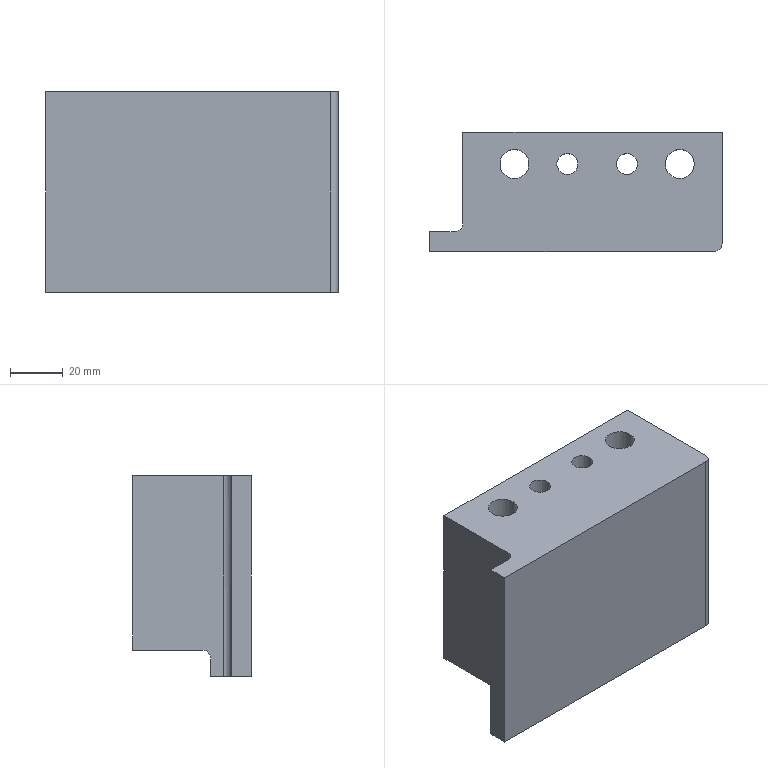Part | NX | features solid 2 | 1 solid | 25 faces | box 110.531 x 45 x 76 mm | volume 282119 mm3 | plane 14 | cylinder 11 | commonest cylinder face diameters 6 x3 8 x2 10.505 x2 11 x2 17 x2
STEP:
#1=CARTESIAN_POINT('',(712.498,169.969,32.999));
#2=VERTEX_POINT('',#1);
#3=CARTESIAN_POINT('',(712.498,166.969,32.999));
#4=VERTEX_POINT('',#3);
#5=CARTESIAN_POINT('',(712.498,196.487,32.999));
#6=DIRECTION('',(0.,-1.,-0.000000517));
#7=VECTOR('',#6,1000.);
#8=LINE('',#5,#7);
#9=EDGE_CURVE('',#2,#4,#8,.T.);
#10=ORIENTED_EDGE('',*,*,#9,.T.);
#11=CARTESIAN_POINT('',(709.498,163.969,32.999));
#12=VERTEX_POINT('',#11);
#13=CARTESIAN_POINT('',(709.498,166.969,32.999));
#14=DIRECTION('',(0.000000053,-0.000000517,1.));
#15=DIRECTION('',(0.01202,0.9999,0.000000516));
#16=AXIS2_PLACEMENT_3D('',#13,#14,#15);
#17=ELLIPSE('',#16,3.,3.);
#18=EDGE_CURVE('',#4,#12,#17,.F.);
#19=ORIENTED_EDGE('',*,*,#18,.T.);
#20=CARTESIAN_POINT('',(699.977,163.969,32.999));
#21=VERTEX_POINT('',#20);
#22=CARTESIAN_POINT('',(704.737,163.969,32.999));
#23=DIRECTION('',(1.,0.,-0.000000053));
#24=VECTOR('',#23,1000.);
#25=LINE('',#22,#24);
#26=EDGE_CURVE('',#12,#21,#25,.F.);
#27=ORIENTED_EDGE('',*,*,#26,.T.);
#28=CARTESIAN_POINT('',(699.977,156.487,32.999));
#29=VERTEX_POINT('',#28);
#30=CARTESIAN_POINT('',(699.977,196.487,32.999));
#31=DIRECTION('',(0.,-1.,-0.000000517));
#32=VECTOR('',#31,1000.);
#33=LINE('',#30,#32);
#34=EDGE_CURVE('',#29,#21,#33,.F.);
#35=ORIENTED_EDGE('',*,*,#34,.F.);
#36=CARTESIAN_POINT('',(807.509,156.487,32.999));
#37=VERTEX_POINT('',#36);
#38=CARTESIAN_POINT('',(699.977,156.487,32.999));
#39=DIRECTION('',(-1.,0.,0.000000053));
#40=VECTOR('',#39,1000.);
#41=LINE('',#38,#40);
#42=EDGE_CURVE('',#29,#37,#41,.F.);
#43=ORIENTED_EDGE('',*,*,#42,.T.);
#44=CARTESIAN_POINT('',(810.509,159.487,32.999));
#45=VERTEX_POINT('',#44);
#46=CARTESIAN_POINT('',(807.509,159.487,32.999));
#47=DIRECTION('',(-0.000000053,0.000000517,-1.));
#48=DIRECTION('',(0.,-1.,-0.000000517));
#49=AXIS2_PLACEMENT_3D('',#46,#47,#48);
#50=CIRCLE('',#49,3.);
#51=EDGE_CURVE('',#45,#37,#50,.T.);
#52=ORIENTED_EDGE('',*,*,#51,.F.);
#53=CARTESIAN_POINT('',(810.509,201.487,32.999));
#54=VERTEX_POINT('',#53);
#55=CARTESIAN_POINT('',(810.509,186.487,32.999));
#56=DIRECTION('',(0.,1.,0.000000517));
#57=VECTOR('',#56,1000.);
#58=LINE('',#55,#57);
#59=EDGE_CURVE('',#54,#45,#58,.F.);
#60=ORIENTED_EDGE('',*,*,#59,.F.);
#61=CARTESIAN_POINT('',(712.498,201.487,32.999));
#62=VERTEX_POINT('',#61);
#63=CARTESIAN_POINT('',(699.977,201.487,32.999));
#64=DIRECTION('',(-1.,0.,0.000000053));
#65=VECTOR('',#64,1000.);
#66=LINE('',#63,#65);
#67=EDGE_CURVE('',#62,#54,#66,.F.);
#68=ORIENTED_EDGE('',*,*,#67,.F.);
#69=CARTESIAN_POINT('',(712.498,196.487,32.999));
#70=DIRECTION('',(0.,1.,0.000000517));
#71=VECTOR('',#70,1000.);
#72=LINE('',#69,#71);
#73=EDGE_CURVE('',#62,#2,#72,.F.);
#74=ORIENTED_EDGE('',*,*,#73,.T.);
#75=EDGE_LOOP('',(#10,#19,#27,#35,#43,#52,#60,#68,#74));
#76=FACE_BOUND('',#75,.T.);
#77=CARTESIAN_POINT('',(794.509,183.987,32.999));
#78=VERTEX_POINT('',#77);
#79=CARTESIAN_POINT('',(794.509,189.487,32.999));
#80=DIRECTION('',(0.000000053,-0.000000517,1.));
#81=DIRECTION('',(0.,-1.,-0.000000517));
#82=AXIS2_PLACEMENT_3D('',#79,#80,#81);
#83=CIRCLE('',#82,5.5);
#84=EDGE_CURVE('',#78,#78,#83,.T.);
#85=ORIENTED_EDGE('',*,*,#84,.F.);
#86=EDGE_LOOP('',(#85));
#87=FACE_BOUND('',#86,.T.);
#88=CARTESIAN_POINT('',(731.977,183.987,32.999));
#89=VERTEX_POINT('',#88);
#90=CARTESIAN_POINT('',(731.977,189.487,32.999));
#91=DIRECTION('',(0.000000053,-0.000000517,1.));
#92=DIRECTION('',(0.,-1.,-0.000000517));
#93=AXIS2_PLACEMENT_3D('',#90,#91,#92);
#94=CIRCLE('',#93,5.5);
#95=EDGE_CURVE('',#89,#89,#94,.T.);
#96=ORIENTED_EDGE('',*,*,#95,.F.);
#97=EDGE_LOOP('',(#96));
#98=FACE_BOUND('',#97,.T.);
#99=CARTESIAN_POINT('',(774.509,193.487,32.999));
#100=VERTEX_POINT('',#99);
#101=CARTESIAN_POINT('',(774.509,189.487,32.999));
#102=DIRECTION('',(0.000000053,-0.000000517,1.));
#103=DIRECTION('',(0.,1.,0.000000517));
#104=AXIS2_PLACEMENT_3D('',#101,#102,#103);
#105=CIRCLE('',#104,4.);
#106=EDGE_CURVE('',#100,#100,#105,.T.);
#107=ORIENTED_EDGE('',*,*,#106,.F.);
#108=EDGE_LOOP('',(#107));
#109=FACE_BOUND('',#108,.T.);
#110=CARTESIAN_POINT('',(751.977,193.487,32.999));
#111=VERTEX_POINT('',#110);
#112=CARTESIAN_POINT('',(751.977,189.487,32.999));
#113=DIRECTION('',(0.000000053,-0.000000517,1.));
#114=DIRECTION('',(0.,1.,0.000000517));
#115=AXIS2_PLACEMENT_3D('',#112,#113,#114);
#116=CIRCLE('',#115,4.);
#117=EDGE_CURVE('',#111,#111,#116,.T.);
#118=ORIENTED_EDGE('',*,*,#117,.F.);
#119=EDGE_LOOP('',(#118));
#120=FACE_BOUND('',#119,.T.);
#121=CARTESIAN_POINT('',(699.977,196.487,32.999));
#122=DIRECTION('',(0.000000053,-0.000000517,1.));
#123=DIRECTION('',(1.,0.,-0.000000053));
#124=AXIS2_PLACEMENT_3D('',#121,#122,#123);
#125=PLANE('',#124);
#126=ADVANCED_FACE('',(#76,#87,#98,#109,#120),#125,.T.);
#127=CARTESIAN_POINT('',(794.509,197.987,-33.001));
#128=VERTEX_POINT('',#127);
#129=CARTESIAN_POINT('',(794.509,189.487,-33.001));
#130=DIRECTION('',(-0.000000053,0.000000517,-1.));
#131=DIRECTION('',(0.,1.,0.000000517));
#132=AXIS2_PLACEMENT_3D('',#129,#130,#131);
#133=CIRCLE('',#132,8.5);
#134=EDGE_CURVE('',#128,#128,#133,.F.);
#135=ORIENTED_EDGE('',*,*,#134,.T.);
#136=EDGE_LOOP('',(#135));
#137=FACE_BOUND('',#136,.T.);
#138=CARTESIAN_POINT('',(774.509,184.234,-33.001));
#139=VERTEX_POINT('',#138);
#140=CARTESIAN_POINT('',(773.441,184.308,-33.001));
#141=CARTESIAN_POINT('',(774.473,184.201,-33.001));
#142=CARTESIAN_POINT('',(775.504,184.297,-33.001));
#143=CARTESIAN_POINT('',(776.482,184.583,-33.001));
#144=CARTESIAN_POINT('',(777.4,185.061,-33.001));
#145=CARTESIAN_POINT('',(778.208,185.71,-33.001));
#146=CARTESIAN_POINT('',(778.873,186.505,-33.001));
#147=CARTESIAN_POINT('',(779.371,187.413,-33.001));
#148=CARTESIAN_POINT('',(779.682,188.402,-33.001));
#149=CARTESIAN_POINT('',(779.795,189.432,-33.001));
#150=CARTESIAN_POINT('',(779.704,190.464,-33.001));
#151=CARTESIAN_POINT('',(779.413,191.459,-33.001));
#152=CARTESIAN_POINT('',(778.934,192.378,-33.001));
#153=CARTESIAN_POINT('',(778.285,193.186,-33.001));
#154=CARTESIAN_POINT('',(777.491,193.852,-33.001));
#155=CARTESIAN_POINT('',(776.582,194.35,-33.001));
#156=CARTESIAN_POINT('',(775.594,194.661,-33.001));
#157=CARTESIAN_POINT('',(774.563,194.773,-33.001));
#158=CARTESIAN_POINT('',(773.531,194.682,-33.001));
#159=CARTESIAN_POINT('',(772.536,194.392,-33.001));
#160=CARTESIAN_POINT('',(771.617,193.913,-33.001));
#161=CARTESIAN_POINT('',(770.81,193.264,-33.001));
#162=CARTESIAN_POINT('',(770.144,192.469,-33.001));
#163=CARTESIAN_POINT('',(769.646,191.561,-33.001));
#164=CARTESIAN_POINT('',(769.335,190.572,-33.001));
#165=CARTESIAN_POINT('',(769.223,189.542,-33.001));
#166=CARTESIAN_POINT('',(769.313,188.509,-33.001));
#167=CARTESIAN_POINT('',(769.604,187.515,-33.001));
#168=CARTESIAN_POINT('',(770.083,186.596,-33.001));
#169=CARTESIAN_POINT('',(770.732,185.788,-33.001));
#170=CARTESIAN_POINT('',(771.526,185.122,-33.001));
#171=CARTESIAN_POINT('',(772.435,184.624,-33.001));
#172=CARTESIAN_POINT('',(773.441,184.308,-33.001));
#173=CARTESIAN_POINT('',(774.473,184.201,-33.001));
#174=CARTESIAN_POINT('',(775.504,184.297,-33.001));
#175=B_SPLINE_CURVE_WITH_KNOTS('',3,(#140,#141,#142,#143,#144,#145,#146,#147,#148,#149,#150,#151,#152,#153,#154,#155,#156,#157,#158,#159,#160,#161,#162,#163,#164,#165,#166,#167,#168,#169,#170,#171,#172,#173,#174),.UNSPECIFIED.,.T.,.F.,(1,1,1,1,1,1,1,1,1,1,1,1,1,1,1,1,1,1,1,1,1,1,1,1,1,1,1,1,1,1,1,1,1,1,1,1,1,1,1),(-0.09539,-0.06414,-0.03289,0.,0.02969,0.06086,0.09211,0.1234,0.1546,0.1859,0.2171,0.2484,0.2796,0.3109,0.3421,0.3734,0.4046,0.4359,0.4671,0.4984,0.5296,0.5609,0.5921,0.6234,0.6546,0.6859,0.7171,0.7484,0.7796,0.8109,0.8421,0.8734,0.9046,0.9359,0.9671,1.,1.03,1.061,1.092),.UNSPECIFIED.);
#176=EDGE_CURVE('',#139,#139,#175,.T.);
#177=ORIENTED_EDGE('',*,*,#176,.T.);
#178=EDGE_LOOP('',(#177));
#179=FACE_BOUND('',#178,.T.);
#180=CARTESIAN_POINT('',(751.977,184.234,-33.001));
#181=VERTEX_POINT('',#180);
#182=CARTESIAN_POINT('',(750.91,184.308,-33.001));
#183=CARTESIAN_POINT('',(751.942,184.201,-33.001));
#184=CARTESIAN_POINT('',(752.973,184.297,-33.001));
#185=CARTESIAN_POINT('',(753.95,184.583,-33.001));
#186=CARTESIAN_POINT('',(754.869,185.061,-33.001));
#187=CARTESIAN_POINT('',(755.676,185.71,-33.001));
#188=CARTESIAN_POINT('',(756.342,186.505,-33.001));
#189=CARTESIAN_POINT('',(756.84,187.413,-33.001));
#190=CARTESIAN_POINT('',(757.151,188.402,-33.001));
#191=CARTESIAN_POINT('',(757.263,189.432,-33.001));
#192=CARTESIAN_POINT('',(757.172,190.464,-33.001));
#193=CARTESIAN_POINT('',(756.882,191.459,-33.001));
#194=CARTESIAN_POINT('',(756.403,192.378,-33.001));
#195=CARTESIAN_POINT('',(755.754,193.186,-33.001));
#196=CARTESIAN_POINT('',(754.96,193.852,-33.001));
#197=CARTESIAN_POINT('',(754.051,194.35,-33.001));
#198=CARTESIAN_POINT('',(753.062,194.661,-33.001));
#199=CARTESIAN_POINT('',(752.032,194.773,-33.001));
#200=CARTESIAN_POINT('',(751.,194.682,-33.001));
#201=CARTESIAN_POINT('',(750.005,194.392,-33.001));
#202=CARTESIAN_POINT('',(749.086,193.913,-33.001));
#203=CARTESIAN_POINT('',(748.278,193.264,-33.001));
#204=CARTESIAN_POINT('',(747.613,192.469,-33.001));
#205=CARTESIAN_POINT('',(747.115,191.561,-33.001));
#206=CARTESIAN_POINT('',(746.803,190.572,-33.001));
#207=CARTESIAN_POINT('',(746.691,189.542,-33.001));
#208=CARTESIAN_POINT('',(746.782,188.51,-33.001));
#209=CARTESIAN_POINT('',(747.073,187.515,-33.001));
#210=CARTESIAN_POINT('',(747.552,186.596,-33.001));
#211=CARTESIAN_POINT('',(748.201,185.788,-33.001));
#212=CARTESIAN_POINT('',(748.995,185.122,-33.001));
#213=CARTESIAN_POINT('',(749.904,184.624,-33.001));
#214=CARTESIAN_POINT('',(750.91,184.308,-33.001));
#215=CARTESIAN_POINT('',(751.942,184.201,-33.001));
#216=CARTESIAN_POINT('',(752.973,184.297,-33.001));
#217=B_SPLINE_CURVE_WITH_KNOTS('',3,(#182,#183,#184,#185,#186,#187,#188,#189,#190,#191,#192,#193,#194,#195,#196,#197,#198,#199,#200,#201,#202,#203,#204,#205,#206,#207,#208,#209,#210,#211,#212,#213,#214,#215,#216),.UNSPECIFIED.,.T.,.F.,(1,1,1,1,1,1,1,1,1,1,1,1,1,1,1,1,1,1,1,1,1,1,1,1,1,1,1,1,1,1,1,1,1,1,1,1,1,1,1),(-0.09539,-0.06414,-0.03289,0.,0.02969,0.06086,0.09211,0.1234,0.1546,0.1859,0.2171,0.2484,0.2796,0.3109,0.3421,0.3734,0.4046,0.4359,0.4671,0.4984,0.5296,0.5609,0.5921,0.6234,0.6546,0.6859,0.7171,0.7484,0.7796,0.8109,0.8421,0.8734,0.9046,0.9359,0.9671,1.,1.03,1.061,1.092),.UNSPECIFIED.);
#218=EDGE_CURVE('',#181,#181,#217,.T.);
#219=ORIENTED_EDGE('',*,*,#218,.T.);
#220=EDGE_LOOP('',(#219));
#221=FACE_BOUND('',#220,.T.);
#222=CARTESIAN_POINT('',(731.977,197.987,-33.001));
#223=VERTEX_POINT('',#222);
#224=CARTESIAN_POINT('',(731.977,189.487,-33.001));
#225=DIRECTION('',(-0.000000053,0.000000517,-1.));
#226=DIRECTION('',(0.,1.,0.000000517));
#227=AXIS2_PLACEMENT_3D('',#224,#225,#226);
#228=CIRCLE('',#227,8.5);
#229=EDGE_CURVE('',#223,#223,#228,.F.);
#230=ORIENTED_EDGE('',*,*,#229,.T.);
#231=EDGE_LOOP('',(#230));
#232=FACE_BOUND('',#231,.T.);
#233=CARTESIAN_POINT('',(810.509,201.487,-33.001));
#234=VERTEX_POINT('',#233);
#235=CARTESIAN_POINT('',(810.509,174.969,-33.001));
#236=VERTEX_POINT('',#235);
#237=CARTESIAN_POINT('',(810.509,186.487,-33.001));
#238=DIRECTION('',(0.,-1.,-0.000000517));
#239=VECTOR('',#238,1000.);
#240=LINE('',#237,#239);
#241=EDGE_CURVE('',#234,#236,#240,.T.);
#242=ORIENTED_EDGE('',*,*,#241,.T.);
#243=CARTESIAN_POINT('',(712.498,174.969,-33.001));
#244=VERTEX_POINT('',#243);
#245=CARTESIAN_POINT('',(712.498,174.969,-33.001));
#246=DIRECTION('',(1.,0.,-0.000000053));
#247=VECTOR('',#246,1000.);
#248=LINE('',#245,#247);
#249=EDGE_CURVE('',#236,#244,#248,.F.);
#250=ORIENTED_EDGE('',*,*,#249,.T.);
#251=CARTESIAN_POINT('',(712.498,201.487,-33.001));
#252=VERTEX_POINT('',#251);
#253=CARTESIAN_POINT('',(712.498,119.199,-33.001));
#254=DIRECTION('',(0.,-1.,-0.000000517));
#255=VECTOR('',#254,1000.);
#256=LINE('',#253,#255);
#257=EDGE_CURVE('',#252,#244,#256,.T.);
#258=ORIENTED_EDGE('',*,*,#257,.F.);
#259=CARTESIAN_POINT('',(574.977,201.487,-33.001));
#260=DIRECTION('',(-1.,0.,0.000000053));
#261=VECTOR('',#260,1000.);
#262=LINE('',#259,#261);
#263=EDGE_CURVE('',#234,#252,#262,.T.);
#264=ORIENTED_EDGE('',*,*,#263,.F.);
#265=EDGE_LOOP('',(#242,#250,#258,#264));
#266=FACE_BOUND('',#265,.T.);
#267=CARTESIAN_POINT('',(574.977,119.199,-33.001));
#268=DIRECTION('',(-0.000000053,0.000000517,-1.));
#269=DIRECTION('',(1.,0.,-0.000000053));
#270=AXIS2_PLACEMENT_3D('',#267,#268,#269);
#271=PLANE('',#270);
#272=ADVANCED_FACE('',(#137,#179,#221,#232,#266),#271,.T.);
#273=CARTESIAN_POINT('',(712.498,171.969,-36.001));
#274=VERTEX_POINT('',#273);
#275=CARTESIAN_POINT('',(712.498,171.969,-43.001));
#276=VERTEX_POINT('',#275);
#277=CARTESIAN_POINT('',(712.498,171.969,49.2));
#278=DIRECTION('',(0.,0.000001782,-1.));
#279=VECTOR('',#278,1000.);
#280=LINE('',#277,#279);
#281=EDGE_CURVE('',#274,#276,#280,.T.);
#282=ORIENTED_EDGE('',*,*,#281,.F.);
#283=CARTESIAN_POINT('',(810.509,171.969,-36.001));
#284=VERTEX_POINT('',#283);
#285=CARTESIAN_POINT('',(810.509,171.969,-36.001));
#286=DIRECTION('',(1.,0.,-0.000000053));
#287=VECTOR('',#286,1000.);
#288=LINE('',#285,#287);
#289=EDGE_CURVE('',#274,#284,#288,.T.);
#290=ORIENTED_EDGE('',*,*,#289,.T.);
#291=CARTESIAN_POINT('',(810.509,171.969,-43.001));
#292=VERTEX_POINT('',#291);
#293=CARTESIAN_POINT('',(810.509,171.969,-43.001));
#294=DIRECTION('',(0.000000053,-0.000001782,1.));
#295=VECTOR('',#294,1000.);
#296=LINE('',#293,#295);
#297=EDGE_CURVE('',#292,#284,#296,.T.);
#298=ORIENTED_EDGE('',*,*,#297,.F.);
#299=CARTESIAN_POINT('',(704.737,171.969,-43.001));
#300=DIRECTION('',(-1.,0.,0.000000053));
#301=VECTOR('',#300,1000.);
#302=LINE('',#299,#301);
#303=EDGE_CURVE('',#292,#276,#302,.T.);
#304=ORIENTED_EDGE('',*,*,#303,.T.);
#305=EDGE_LOOP('',(#282,#290,#298,#304));
#306=FACE_BOUND('',#305,.T.);
#307=CARTESIAN_POINT('',(704.737,171.969,-5.001));
#308=DIRECTION('',(0.,1.,0.000001782));
#309=DIRECTION('',(0.,0.000001782,-1.));
#310=AXIS2_PLACEMENT_3D('',#307,#308,#309);
#311=PLANE('',#310);
#312=ADVANCED_FACE('',(#306),#311,.T.);
#313=ORIENTED_EDGE('',*,*,#42,.F.);
#314=CARTESIAN_POINT('',(699.977,156.487,-43.001));
#315=VERTEX_POINT('',#314);
#316=CARTESIAN_POINT('',(699.977,156.487,56.368));
#317=DIRECTION('',(0.000000053,-0.000000517,1.));
#318=VECTOR('',#317,1000.);
#319=LINE('',#316,#318);
#320=EDGE_CURVE('',#29,#315,#319,.F.);
#321=ORIENTED_EDGE('',*,*,#320,.T.);
#322=CARTESIAN_POINT('',(807.509,156.487,-43.001));
#323=VERTEX_POINT('',#322);
#324=CARTESIAN_POINT('',(574.977,156.487,-43.001));
#325=DIRECTION('',(1.,0.,-0.000000053));
#326=VECTOR('',#325,1000.);
#327=LINE('',#324,#326);
#328=EDGE_CURVE('',#315,#323,#327,.T.);
#329=ORIENTED_EDGE('',*,*,#328,.T.);
#330=CARTESIAN_POINT('',(807.509,156.487,56.368));
#331=DIRECTION('',(-0.000000053,0.000000517,-1.));
#332=VECTOR('',#331,1000.);
#333=LINE('',#330,#332);
#334=EDGE_CURVE('',#323,#37,#333,.F.);
#335=ORIENTED_EDGE('',*,*,#334,.T.);
#336=EDGE_LOOP('',(#313,#321,#329,#335));
#337=FACE_BOUND('',#336,.T.);
#338=CARTESIAN_POINT('',(583.446,156.487,56.368));
#339=DIRECTION('',(0.,1.,0.000000517));
#340=DIRECTION('',(-0.000000053,0.000000517,-1.));
#341=AXIS2_PLACEMENT_3D('',#338,#339,#340);
#342=PLANE('',#341);
#343=ADVANCED_FACE('',(#337),#342,.F.);
#344=ORIENTED_EDGE('',*,*,#328,.F.);
#345=CARTESIAN_POINT('',(699.977,163.969,-43.001));
#346=VERTEX_POINT('',#345);
#347=CARTESIAN_POINT('',(699.977,119.199,-43.001));
#348=DIRECTION('',(0.,1.,0.000000517));
#349=VECTOR('',#348,1000.);
#350=LINE('',#347,#349);
#351=EDGE_CURVE('',#346,#315,#350,.F.);
#352=ORIENTED_EDGE('',*,*,#351,.F.);
#353=CARTESIAN_POINT('',(709.498,163.969,-43.001));
#354=VERTEX_POINT('',#353);
#355=CARTESIAN_POINT('',(704.737,163.969,-43.001));
#356=DIRECTION('',(-1.,0.,0.000000053));
#357=VECTOR('',#356,1000.);
#358=LINE('',#355,#357);
#359=EDGE_CURVE('',#354,#346,#358,.T.);
#360=ORIENTED_EDGE('',*,*,#359,.F.);
#361=CARTESIAN_POINT('',(712.498,166.969,-43.001));
#362=VERTEX_POINT('',#361);
#363=CARTESIAN_POINT('',(709.498,166.969,-43.001));
#364=DIRECTION('',(-0.000000053,0.000000517,-1.));
#365=DIRECTION('',(0.01202,0.9999,0.000000516));
#366=AXIS2_PLACEMENT_3D('',#363,#364,#365);
#367=ELLIPSE('',#366,3.,3.);
#368=EDGE_CURVE('',#354,#362,#367,.F.);
#369=ORIENTED_EDGE('',*,*,#368,.T.);
#370=CARTESIAN_POINT('',(712.498,119.199,-43.001));
#371=DIRECTION('',(0.,1.,0.000000517));
#372=VECTOR('',#371,1000.);
#373=LINE('',#370,#372);
#374=EDGE_CURVE('',#362,#276,#373,.T.);
#375=ORIENTED_EDGE('',*,*,#374,.T.);
#376=ORIENTED_EDGE('',*,*,#303,.F.);
#377=CARTESIAN_POINT('',(810.509,159.487,-43.001));
#378=VERTEX_POINT('',#377);
#379=CARTESIAN_POINT('',(810.509,186.487,-43.001));
#380=DIRECTION('',(0.,-1.,-0.000000517));
#381=VECTOR('',#380,1000.);
#382=LINE('',#379,#381);
#383=EDGE_CURVE('',#292,#378,#382,.T.);
#384=ORIENTED_EDGE('',*,*,#383,.T.);
#385=CARTESIAN_POINT('',(807.509,159.487,-43.001));
#386=DIRECTION('',(0.000000053,-0.000000517,1.));
#387=DIRECTION('',(0.,1.,0.000000517));
#388=AXIS2_PLACEMENT_3D('',#385,#386,#387);
#389=CIRCLE('',#388,3.);
#390=EDGE_CURVE('',#378,#323,#389,.F.);
#391=ORIENTED_EDGE('',*,*,#390,.T.);
#392=EDGE_LOOP('',(#344,#352,#360,#369,#375,#376,#384,#391));
#393=FACE_BOUND('',#392,.T.);
#394=CARTESIAN_POINT('',(574.977,119.199,-43.001));
#395=DIRECTION('',(-0.000000053,0.000000517,-1.));
#396=DIRECTION('',(1.,0.,-0.000000053));
#397=AXIS2_PLACEMENT_3D('',#394,#395,#396);
#398=PLANE('',#397);
#399=ADVANCED_FACE('',(#393),#398,.T.);
#400=ORIENTED_EDGE('',*,*,#59,.T.);
#401=CARTESIAN_POINT('',(810.509,159.487,-43.001));
#402=DIRECTION('',(-0.000000053,0.000000517,-1.));
#403=VECTOR('',#402,1000.);
#404=LINE('',#401,#403);
#405=EDGE_CURVE('',#45,#378,#404,.T.);
#406=ORIENTED_EDGE('',*,*,#405,.T.);
#407=ORIENTED_EDGE('',*,*,#383,.F.);
#408=ORIENTED_EDGE('',*,*,#297,.T.);
#409=CARTESIAN_POINT('',(810.509,174.969,-36.001));
#410=DIRECTION('',(1.,0.,-0.000000053));
#411=DIRECTION('',(-0.000000053,0.,-1.));
#412=AXIS2_PLACEMENT_3D('',#409,#410,#411);
#413=CIRCLE('',#412,3.);
#414=EDGE_CURVE('',#284,#236,#413,.F.);
#415=ORIENTED_EDGE('',*,*,#414,.T.);
#416=ORIENTED_EDGE('',*,*,#241,.F.);
#417=CARTESIAN_POINT('',(810.509,201.487,-43.001));
#418=DIRECTION('',(0.000000053,-0.000000517,1.));
#419=VECTOR('',#418,1000.);
#420=LINE('',#417,#419);
#421=EDGE_CURVE('',#54,#234,#420,.F.);
#422=ORIENTED_EDGE('',*,*,#421,.F.);
#423=EDGE_LOOP('',(#400,#406,#407,#408,#415,#416,#422));
#424=FACE_BOUND('',#423,.T.);
#425=CARTESIAN_POINT('',(810.509,186.487,-43.001));
#426=DIRECTION('',(1.,0.,-0.000000053));
#427=DIRECTION('',(0.000000053,-0.000000517,1.));
#428=AXIS2_PLACEMENT_3D('',#425,#426,#427);
#429=PLANE('',#428);
#430=ADVANCED_FACE('',(#424),#429,.T.);
#431=ORIENTED_EDGE('',*,*,#67,.T.);
#432=ORIENTED_EDGE('',*,*,#421,.T.);
#433=ORIENTED_EDGE('',*,*,#263,.T.);
#434=CARTESIAN_POINT('',(712.498,201.487,-43.001));
#435=DIRECTION('',(0.,0.000000517,-1.));
#436=VECTOR('',#435,1000.);
#437=LINE('',#434,#436);
#438=EDGE_CURVE('',#62,#252,#437,.T.);
#439=ORIENTED_EDGE('',*,*,#438,.F.);
#440=EDGE_LOOP('',(#431,#432,#433,#439));
#441=FACE_BOUND('',#440,.T.);
#442=CARTESIAN_POINT('',(699.977,201.487,-43.001));
#443=DIRECTION('',(0.,1.,0.000000517));
#444=DIRECTION('',(-0.000000053,0.000000517,-1.));
#445=AXIS2_PLACEMENT_3D('',#442,#443,#444);
#446=PLANE('',#445);
#447=ADVANCED_FACE('',(#441),#446,.T.);
#448=ORIENTED_EDGE('',*,*,#257,.T.);
#449=CARTESIAN_POINT('',(712.498,174.969,-36.001));
#450=DIRECTION('',(-1.,0.,0.));
#451=DIRECTION('',(0.,-1.,0.));
#452=AXIS2_PLACEMENT_3D('',#449,#450,#451);
#453=CIRCLE('',#452,3.);
#454=EDGE_CURVE('',#244,#274,#453,.F.);
#455=ORIENTED_EDGE('',*,*,#454,.T.);
#456=ORIENTED_EDGE('',*,*,#281,.T.);
#457=ORIENTED_EDGE('',*,*,#374,.F.);
#458=CARTESIAN_POINT('',(712.498,166.969,32.999));
#459=DIRECTION('',(0.,-0.000004945,1.));
#460=VECTOR('',#459,1000.);
#461=LINE('',#458,#460);
#462=EDGE_CURVE('',#362,#4,#461,.T.);
#463=ORIENTED_EDGE('',*,*,#462,.T.);
#464=ORIENTED_EDGE('',*,*,#9,.F.);
#465=ORIENTED_EDGE('',*,*,#73,.F.);
#466=ORIENTED_EDGE('',*,*,#438,.T.);
#467=EDGE_LOOP('',(#448,#455,#456,#457,#463,#464,#465,#466));
#468=FACE_BOUND('',#467,.T.);
#469=CARTESIAN_POINT('',(712.498,185.969,49.2));
#470=DIRECTION('',(-1.,0.,0.));
#471=DIRECTION('',(0.,1.,0.000004363));
#472=AXIS2_PLACEMENT_3D('',#469,#470,#471);
#473=PLANE('',#472);
#474=ADVANCED_FACE('',(#468),#473,.T.);
#475=CARTESIAN_POINT('',(794.509,194.987,7.999));
#476=VERTEX_POINT('',#475);
#477=CARTESIAN_POINT('',(794.509,189.487,7.999));
#478=DIRECTION('',(-0.00000016,0.000000517,-1.));
#479=DIRECTION('',(0.,1.,0.000000517));
#480=AXIS2_PLACEMENT_3D('',#477,#478,#479);
#481=CIRCLE('',#480,5.5);
#482=EDGE_CURVE('',#476,#476,#481,.F.);
#483=ORIENTED_EDGE('',*,*,#482,.F.);
#484=EDGE_LOOP('',(#483));
#485=FACE_BOUND('',#484,.T.);
#486=ORIENTED_EDGE('',*,*,#84,.T.);
#487=EDGE_LOOP('',(#486));
#488=FACE_BOUND('',#487,.T.);
#489=CARTESIAN_POINT('',(794.509,189.487,33.999));
#490=DIRECTION('',(-0.00000016,0.000000517,-1.));
#491=DIRECTION('',(0.,1.,0.000000517));
#492=AXIS2_PLACEMENT_3D('',#489,#490,#491);
#493=CYLINDRICAL_SURFACE('',#492,5.5);
#494=ADVANCED_FACE('',(#485,#488),#493,.F.);
#495=ORIENTED_EDGE('',*,*,#134,.F.);
#496=EDGE_LOOP('',(#495));
#497=FACE_BOUND('',#496,.T.);
#498=CARTESIAN_POINT('',(794.509,197.987,7.999));
#499=VERTEX_POINT('',#498);
#500=CARTESIAN_POINT('',(794.509,189.487,7.999));
#501=DIRECTION('',(-0.00000016,0.000000517,-1.));
#502=DIRECTION('',(0.,1.,0.000000517));
#503=AXIS2_PLACEMENT_3D('',#500,#501,#502);
#504=CIRCLE('',#503,8.5);
#505=EDGE_CURVE('',#499,#499,#504,.T.);
#506=ORIENTED_EDGE('',*,*,#505,.F.);
#507=EDGE_LOOP('',(#506));
#508=FACE_BOUND('',#507,.T.);
#509=CARTESIAN_POINT('',(794.509,189.487,7.999));
#510=DIRECTION('',(-0.00000016,0.000000517,-1.));
#511=DIRECTION('',(0.,1.,0.000000517));
#512=AXIS2_PLACEMENT_3D('',#509,#510,#511);
#513=CYLINDRICAL_SURFACE('',#512,8.5);
#514=ADVANCED_FACE('',(#497,#508),#513,.F.);
#515=ORIENTED_EDGE('',*,*,#482,.T.);
#516=EDGE_LOOP('',(#515));
#517=FACE_BOUND('',#516,.T.);
#518=ORIENTED_EDGE('',*,*,#505,.T.);
#519=EDGE_LOOP('',(#518));
#520=FACE_BOUND('',#519,.T.);
#521=CARTESIAN_POINT('',(794.509,189.487,7.999));
#522=DIRECTION('',(-0.00000016,0.000000517,-1.));
#523=DIRECTION('',(0.,1.,0.000000517));
#524=AXIS2_PLACEMENT_3D('',#521,#522,#523);
#525=PLANE('',#524);
#526=ADVANCED_FACE('',(#517,#520),#525,.T.);
#527=CARTESIAN_POINT('',(778.509,189.487,-13.001));
#528=VERTEX_POINT('',#527);
#529=CARTESIAN_POINT('',(774.509,189.487,-13.001));
#530=DIRECTION('',(0.000000874,-0.000000517,-1.));
#531=DIRECTION('',(1.,0.,0.000000874));
#532=AXIS2_PLACEMENT_3D('',#529,#530,#531);
#533=CIRCLE('',#532,4.);
#534=EDGE_CURVE('',#528,#528,#533,.F.);
#535=ORIENTED_EDGE('',*,*,#534,.F.);
#536=EDGE_LOOP('',(#535));
#537=FACE_BOUND('',#536,.T.);
#538=ORIENTED_EDGE('',*,*,#106,.T.);
#539=EDGE_LOOP('',(#538));
#540=FACE_BOUND('',#539,.T.);
#541=CARTESIAN_POINT('',(774.509,189.487,33.999));
#542=DIRECTION('',(0.000000874,-0.000000517,-1.));
#543=DIRECTION('',(0.,1.,-0.000000517));
#544=AXIS2_PLACEMENT_3D('',#541,#542,#543);
#545=CYLINDRICAL_SURFACE('',#544,4.);
#546=ADVANCED_FACE('',(#537,#540),#545,.F.);
#547=ORIENTED_EDGE('',*,*,#176,.F.);
#548=EDGE_LOOP('',(#547));
#549=FACE_BOUND('',#548,.T.);
#550=CARTESIAN_POINT('',(779.761,189.487,-13.001));
#551=VERTEX_POINT('',#550);
#552=CARTESIAN_POINT('',(774.509,189.487,-13.001));
#553=DIRECTION('',(0.000000874,-0.000000517,-1.));
#554=DIRECTION('',(1.,0.,0.000000874));
#555=AXIS2_PLACEMENT_3D('',#552,#553,#554);
#556=CIRCLE('',#555,5.253);
#557=EDGE_CURVE('',#551,#551,#556,.T.);
#558=ORIENTED_EDGE('',*,*,#557,.F.);
#559=EDGE_LOOP('',(#558));
#560=FACE_BOUND('',#559,.T.);
#561=CARTESIAN_POINT('',(774.509,189.487,-33.001));
#562=DIRECTION('',(0.000000874,-0.000000517,-1.));
#563=DIRECTION('',(0.,1.,-0.000000517));
#564=AXIS2_PLACEMENT_3D('',#561,#562,#563);
#565=CYLINDRICAL_SURFACE('',#564,5.253);
#566=ADVANCED_FACE('',(#549,#560),#565,.F.);
#567=ORIENTED_EDGE('',*,*,#534,.T.);
#568=EDGE_LOOP('',(#567));
#569=FACE_BOUND('',#568,.T.);
#570=ORIENTED_EDGE('',*,*,#557,.T.);
#571=EDGE_LOOP('',(#570));
#572=FACE_BOUND('',#571,.T.);
#573=CARTESIAN_POINT('',(774.509,189.487,-13.001));
#574=DIRECTION('',(0.000000874,-0.000000517,-1.));
#575=DIRECTION('',(0.,1.,-0.000000517));
#576=AXIS2_PLACEMENT_3D('',#573,#574,#575);
#577=PLANE('',#576);
#578=ADVANCED_FACE('',(#569,#572),#577,.T.);
#579=CARTESIAN_POINT('',(751.977,193.487,-13.001));
#580=VERTEX_POINT('',#579);
#581=CARTESIAN_POINT('',(751.977,189.487,-13.001));
#582=DIRECTION('',(-0.000001087,-0.000000517,-1.));
#583=DIRECTION('',(0.,1.,-0.000000517));
#584=AXIS2_PLACEMENT_3D('',#581,#582,#583);
#585=CIRCLE('',#584,4.);
#586=EDGE_CURVE('',#580,#580,#585,.T.);
#587=ORIENTED_EDGE('',*,*,#586,.T.);
#588=EDGE_LOOP('',(#587));
#589=FACE_BOUND('',#588,.T.);
#590=ORIENTED_EDGE('',*,*,#117,.T.);
#591=EDGE_LOOP('',(#590));
#592=FACE_BOUND('',#591,.T.);
#593=CARTESIAN_POINT('',(751.977,189.487,33.999));
#594=DIRECTION('',(-0.000001087,-0.000000517,-1.));
#595=DIRECTION('',(0.,1.,-0.000000517));
#596=AXIS2_PLACEMENT_3D('',#593,#594,#595);
#597=CYLINDRICAL_SURFACE('',#596,4.);
#598=ADVANCED_FACE('',(#589,#592),#597,.F.);
#599=ORIENTED_EDGE('',*,*,#218,.F.);
#600=EDGE_LOOP('',(#599));
#601=FACE_BOUND('',#600,.T.);
#602=CARTESIAN_POINT('',(746.725,189.487,-13.001));
#603=VERTEX_POINT('',#602);
#604=CARTESIAN_POINT('',(751.977,189.487,-13.001));
#605=DIRECTION('',(-0.000001087,-0.000000517,-1.));
#606=DIRECTION('',(-1.,0.,0.000001087));
#607=AXIS2_PLACEMENT_3D('',#604,#605,#606);
#608=CIRCLE('',#607,5.253);
#609=EDGE_CURVE('',#603,#603,#608,.F.);
#610=ORIENTED_EDGE('',*,*,#609,.T.);
#611=EDGE_LOOP('',(#610));
#612=FACE_BOUND('',#611,.T.);
#613=CARTESIAN_POINT('',(751.977,189.487,-33.001));
#614=DIRECTION('',(-0.000001087,-0.000000517,-1.));
#615=DIRECTION('',(0.,1.,-0.000000517));
#616=AXIS2_PLACEMENT_3D('',#613,#614,#615);
#617=CYLINDRICAL_SURFACE('',#616,5.253);
#618=ADVANCED_FACE('',(#601,#612),#617,.F.);
#619=ORIENTED_EDGE('',*,*,#586,.F.);
#620=EDGE_LOOP('',(#619));
#621=FACE_BOUND('',#620,.T.);
#622=ORIENTED_EDGE('',*,*,#609,.F.);
#623=EDGE_LOOP('',(#622));
#624=FACE_BOUND('',#623,.T.);
#625=CARTESIAN_POINT('',(751.977,189.487,-13.001));
#626=DIRECTION('',(-0.000001087,-0.000000517,-1.));
#627=DIRECTION('',(0.,1.,-0.000000517));
#628=AXIS2_PLACEMENT_3D('',#625,#626,#627);
#629=PLANE('',#628);
#630=ADVANCED_FACE('',(#621,#624),#629,.T.);
#631=CARTESIAN_POINT('',(731.977,194.987,7.999));
#632=VERTEX_POINT('',#631);
#633=CARTESIAN_POINT('',(731.977,189.487,7.999));
#634=DIRECTION('',(-0.000000053,0.000000517,-1.));
#635=DIRECTION('',(0.,1.,0.000000517));
#636=AXIS2_PLACEMENT_3D('',#633,#634,#635);
#637=CIRCLE('',#636,5.5);
#638=EDGE_CURVE('',#632,#632,#637,.T.);
#639=ORIENTED_EDGE('',*,*,#638,.T.);
#640=EDGE_LOOP('',(#639));
#641=FACE_BOUND('',#640,.T.);
#642=ORIENTED_EDGE('',*,*,#95,.T.);
#643=EDGE_LOOP('',(#642));
#644=FACE_BOUND('',#643,.T.);
#645=CARTESIAN_POINT('',(731.977,189.487,33.999));
#646=DIRECTION('',(-0.000000053,0.000000517,-1.));
#647=DIRECTION('',(0.,1.,0.000000517));
#648=AXIS2_PLACEMENT_3D('',#645,#646,#647);
#649=CYLINDRICAL_SURFACE('',#648,5.5);
#650=ADVANCED_FACE('',(#641,#644),#649,.F.);
#651=ORIENTED_EDGE('',*,*,#229,.F.);
#652=EDGE_LOOP('',(#651));
#653=FACE_BOUND('',#652,.T.);
#654=CARTESIAN_POINT('',(731.977,197.987,7.999));
#655=VERTEX_POINT('',#654);
#656=CARTESIAN_POINT('',(731.977,189.487,7.999));
#657=DIRECTION('',(-0.000000053,0.000000517,-1.));
#658=DIRECTION('',(0.,1.,0.000000517));
#659=AXIS2_PLACEMENT_3D('',#656,#657,#658);
#660=CIRCLE('',#659,8.5);
#661=EDGE_CURVE('',#655,#655,#660,.F.);
#662=ORIENTED_EDGE('',*,*,#661,.T.);
#663=EDGE_LOOP('',(#662));
#664=FACE_BOUND('',#663,.T.);
#665=CARTESIAN_POINT('',(731.977,189.487,7.999));
#666=DIRECTION('',(-0.000000053,0.000000517,-1.));
#667=DIRECTION('',(0.,1.,0.000000517));
#668=AXIS2_PLACEMENT_3D('',#665,#666,#667);
#669=CYLINDRICAL_SURFACE('',#668,8.5);
#670=ADVANCED_FACE('',(#653,#664),#669,.F.);
#671=ORIENTED_EDGE('',*,*,#638,.F.);
#672=EDGE_LOOP('',(#671));
#673=FACE_BOUND('',#672,.T.);
#674=ORIENTED_EDGE('',*,*,#661,.F.);
#675=EDGE_LOOP('',(#674));
#676=FACE_BOUND('',#675,.T.);
#677=CARTESIAN_POINT('',(731.977,189.487,7.999));
#678=DIRECTION('',(-0.000000053,0.000000517,-1.));
#679=DIRECTION('',(0.,1.,0.000000517));
#680=AXIS2_PLACEMENT_3D('',#677,#678,#679);
#681=PLANE('',#680);
#682=ADVANCED_FACE('',(#673,#676),#681,.T.);
#683=ORIENTED_EDGE('',*,*,#51,.T.);
#684=ORIENTED_EDGE('',*,*,#334,.F.);
#685=ORIENTED_EDGE('',*,*,#390,.F.);
#686=ORIENTED_EDGE('',*,*,#405,.F.);
#687=EDGE_LOOP('',(#683,#684,#685,#686));
#688=FACE_BOUND('',#687,.T.);
#689=CARTESIAN_POINT('',(807.509,159.487,-43.001));
#690=DIRECTION('',(-0.000000053,0.000000517,-1.));
#691=DIRECTION('',(0.,1.,0.000000517));
#692=AXIS2_PLACEMENT_3D('',#689,#690,#691);
#693=CYLINDRICAL_SURFACE('',#692,3.);
#694=ADVANCED_FACE('',(#688),#693,.T.);
#695=ORIENTED_EDGE('',*,*,#351,.T.);
#696=ORIENTED_EDGE('',*,*,#320,.F.);
#697=ORIENTED_EDGE('',*,*,#34,.T.);
#698=CARTESIAN_POINT('',(699.977,163.969,-5.001));
#699=DIRECTION('',(-0.000000053,0.000004945,-1.));
#700=VECTOR('',#699,1000.);
#701=LINE('',#698,#700);
#702=EDGE_CURVE('',#21,#346,#701,.T.);
#703=ORIENTED_EDGE('',*,*,#702,.T.);
#704=EDGE_LOOP('',(#695,#696,#697,#703));
#705=FACE_BOUND('',#704,.T.);
#706=CARTESIAN_POINT('',(699.977,156.487,-43.001));
#707=DIRECTION('',(1.,0.,-0.000000053));
#708=DIRECTION('',(0.000000053,-0.000001034,1.));
#709=AXIS2_PLACEMENT_3D('',#706,#707,#708);
#710=PLANE('',#709);
#711=ADVANCED_FACE('',(#705),#710,.F.);
#712=ORIENTED_EDGE('',*,*,#26,.F.);
#713=CARTESIAN_POINT('',(709.498,163.969,-43.001));
#714=DIRECTION('',(0.,-0.000004945,1.));
#715=VECTOR('',#714,1000.);
#716=LINE('',#713,#715);
#717=EDGE_CURVE('',#12,#354,#716,.F.);
#718=ORIENTED_EDGE('',*,*,#717,.T.);
#719=ORIENTED_EDGE('',*,*,#359,.T.);
#720=ORIENTED_EDGE('',*,*,#702,.F.);
#721=EDGE_LOOP('',(#712,#718,#719,#720));
#722=FACE_BOUND('',#721,.T.);
#723=CARTESIAN_POINT('',(704.737,163.969,-5.001));
#724=DIRECTION('',(0.,1.,0.000004945));
#725=DIRECTION('',(0.,0.000004945,-1.));
#726=AXIS2_PLACEMENT_3D('',#723,#724,#725);
#727=PLANE('',#726);
#728=ADVANCED_FACE('',(#722),#727,.T.);
#729=ORIENTED_EDGE('',*,*,#368,.F.);
#730=ORIENTED_EDGE('',*,*,#717,.F.);
#731=ORIENTED_EDGE('',*,*,#18,.F.);
#732=ORIENTED_EDGE('',*,*,#462,.F.);
#733=EDGE_LOOP('',(#729,#730,#731,#732));
#734=FACE_BOUND('',#733,.T.);
#735=CARTESIAN_POINT('',(709.498,166.969,49.2));
#736=DIRECTION('',(0.,0.000004945,-1.));
#737=DIRECTION('',(0.,-1.,-0.000004945));
#738=AXIS2_PLACEMENT_3D('',#735,#736,#737);
#739=CYLINDRICAL_SURFACE('',#738,3.);
#740=ADVANCED_FACE('',(#734),#739,.F.);
#741=ORIENTED_EDGE('',*,*,#454,.F.);
#742=ORIENTED_EDGE('',*,*,#249,.F.);
#743=ORIENTED_EDGE('',*,*,#414,.F.);
#744=ORIENTED_EDGE('',*,*,#289,.F.);
#745=EDGE_LOOP('',(#741,#742,#743,#744));
#746=FACE_BOUND('',#745,.T.);
#747=CARTESIAN_POINT('',(704.737,174.969,-36.001));
#748=DIRECTION('',(-1.,0.,0.000000053));
#749=DIRECTION('',(0.000000053,0.,1.));
#750=AXIS2_PLACEMENT_3D('',#747,#748,#749);
#751=CYLINDRICAL_SURFACE('',#750,3.);
#752=ADVANCED_FACE('',(#746),#751,.F.);
#753=CLOSED_SHELL('',(#126,#272,#312,#343,#399,#430,#447,#474,#494,#514,#526,#546,#566,#578,#598,#618,#630,#650,#670,#682,#694,#711,#728,#740,#752));
#754=MANIFOLD_SOLID_BREP('',#753);
#755=(LENGTH_UNIT()NAMED_UNIT(*)SI_UNIT(.MILLI.,.METRE.));
#756=UNCERTAINTY_MEASURE_WITH_UNIT(LENGTH_MEASURE(0.0508),#755,'','');
#757=(NAMED_UNIT(*)PLANE_ANGLE_UNIT()SI_UNIT($,.RADIAN.));
#758=(NAMED_UNIT(*)SI_UNIT($,.STERADIAN.)SOLID_ANGLE_UNIT());
#759=(GEOMETRIC_REPRESENTATION_CONTEXT(3)GLOBAL_UNCERTAINTY_ASSIGNED_CONTEXT((#756))GLOBAL_UNIT_ASSIGNED_CONTEXT((#755,#757,#758))REPRESENTATION_CONTEXT('',''));
#760=ADVANCED_BREP_SHAPE_REPRESENTATION('',(#754),#759);